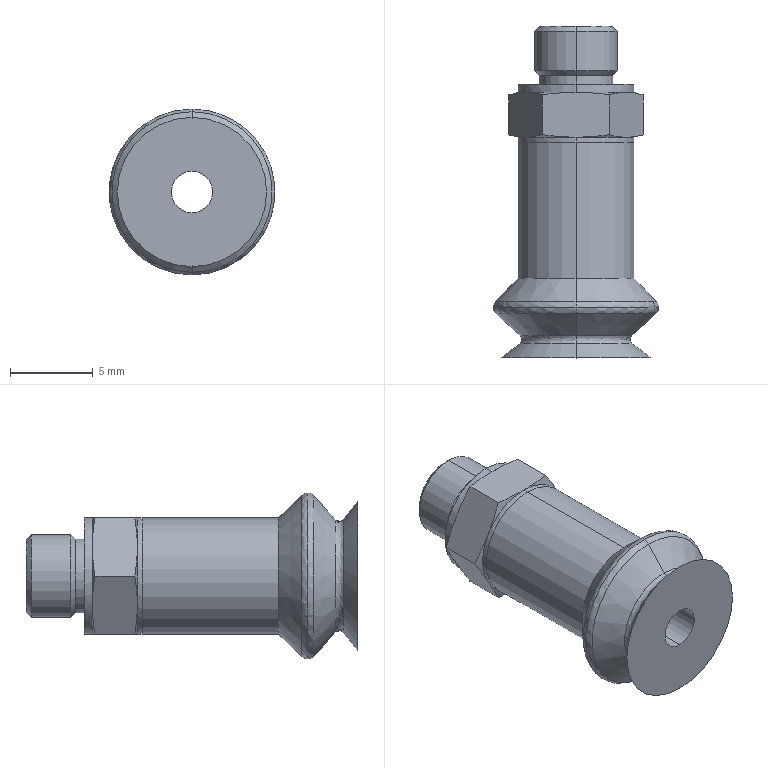Part | STEP file | Vacuum suction cup ZPT08BS-A5_longitudinal vacuum outlet type_no buffer_bellows type | 2 solids | 54 faces | box 10 x 20 x 10 mm | volume 691.38 mm3 | cone 22 | cylinder 14 | plane 12 | spline 6 | commonest cylinder face diameters 7 x6 2.5 x4 4.46 x2 5 x2